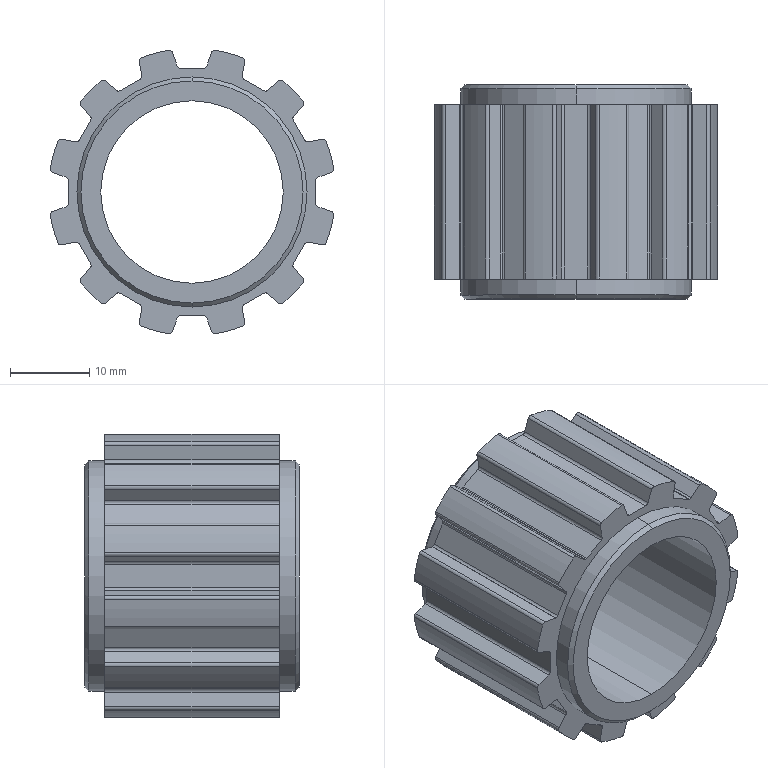Part | SolidWorks | features Cut 2, Chamfer 1, Extrusion 1 | 1 solid | 120 faces | box 35.736 x 27 x 35.736 mm | volume 11879 mm3 | cylinder 76 | plane 40 | cone 4 | commonest cylinder face diameters 0.8 x58 36.2 x12 29 x4 23 x2